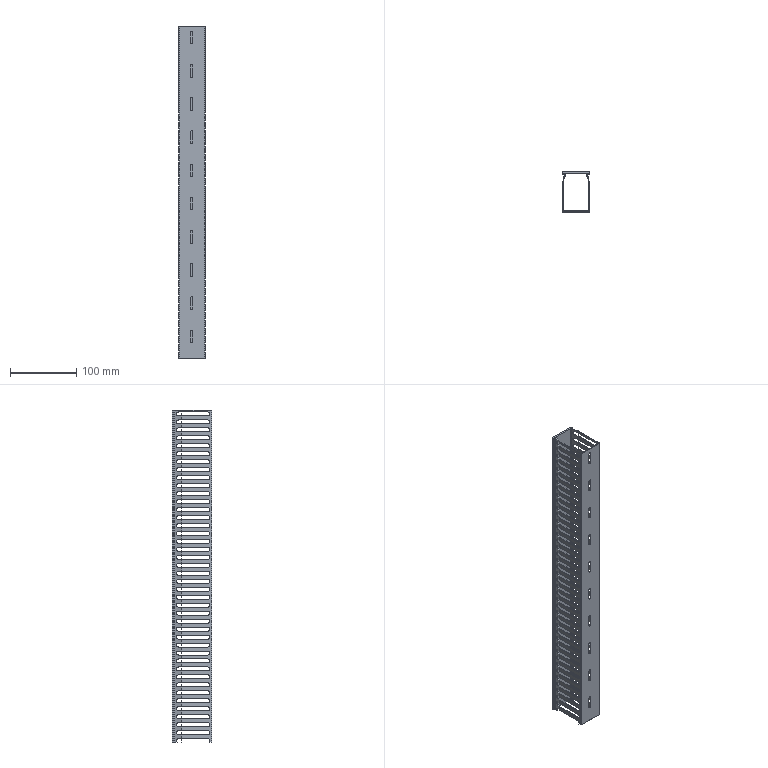Part | STEP file | cable tray 40-60-490 | 1 solid | 628 faces | box 40 x 60 x 500 mm | volume 93421 mm3 | cylinder 373 | plane 255 | commonest cylinder face diameters 6 x252 1.6 x91 4.2 x30